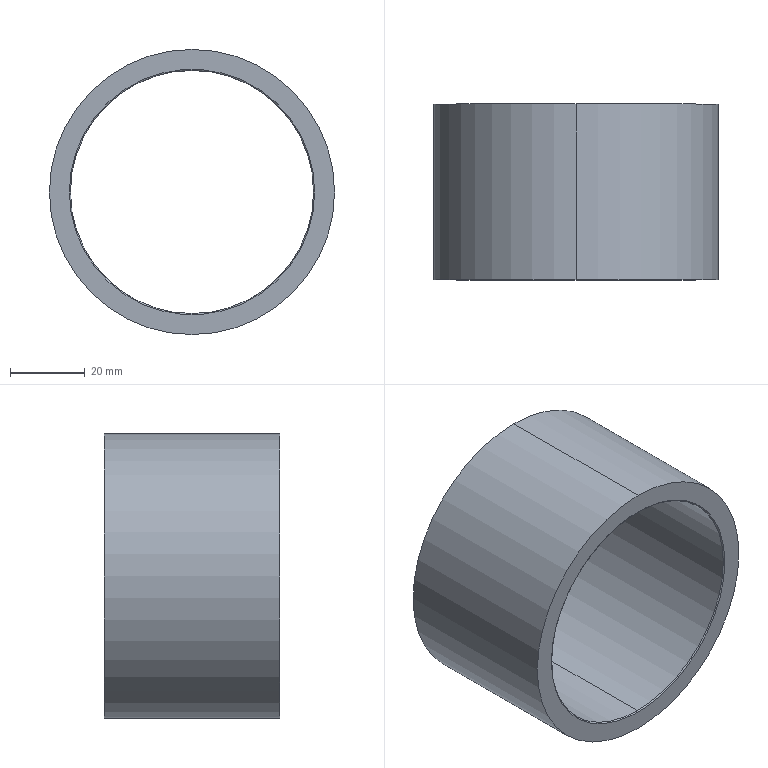Part | SolidWorks | features BaseBody 1 | 1 solid | 10 faces | box 76.25 x 47 x 76.25 mm | volume 58650 mm3 | cylinder 4 | torus 4 | plane 2 | commonest cylinder face diameters 65 x2 76.25 x2
STEP:
#1=CARTESIAN_POINT('',(-2100.15,744.069,-1577.624));
#2=VERTEX_POINT('',#1);
#3=CARTESIAN_POINT('',(-2165.75,744.069,-1577.624));
#4=VERTEX_POINT('',#3);
#5=CARTESIAN_POINT('',(-2132.95,744.069,-1577.624));
#6=DIRECTION('',(0.,-1.,0.));
#7=DIRECTION('',(0.,0.,1.));
#8=AXIS2_PLACEMENT_3D('',#5,#6,#7);
#9=CIRCLE('',#8,32.8);
#10=EDGE_CURVE('',#2,#4,#9,.T.);
#11=ORIENTED_EDGE('',*,*,#10,.F.);
#12=CARTESIAN_POINT('',(-2132.95,744.069,-1577.624));
#13=DIRECTION('',(0.,-1.,0.));
#14=DIRECTION('',(-1.,0.,0.));
#15=AXIS2_PLACEMENT_3D('',#12,#13,#14);
#16=CIRCLE('',#15,32.8);
#17=EDGE_CURVE('',#4,#2,#16,.T.);
#18=ORIENTED_EDGE('',*,*,#17,.F.);
#19=EDGE_LOOP('',(#11,#18));
#20=FACE_BOUND('',#19,.T.);
#21=CARTESIAN_POINT('',(-2132.95,744.069,-1539.499));
#22=VERTEX_POINT('',#21);
#23=CARTESIAN_POINT('',(-2132.95,744.069,-1615.749));
#24=VERTEX_POINT('',#23);
#25=CARTESIAN_POINT('',(-2132.95,744.069,-1577.624));
#26=DIRECTION('',(0.,-1.,0.));
#27=DIRECTION('',(0.,0.,1.));
#28=AXIS2_PLACEMENT_3D('',#25,#26,#27);
#29=CIRCLE('',#28,38.125);
#30=EDGE_CURVE('',#22,#24,#29,.T.);
#31=ORIENTED_EDGE('',*,*,#30,.T.);
#32=CARTESIAN_POINT('',(-2132.95,744.069,-1577.624));
#33=DIRECTION('',(0.,-1.,0.));
#34=DIRECTION('',(0.,0.,-1.));
#35=AXIS2_PLACEMENT_3D('',#32,#33,#34);
#36=CIRCLE('',#35,38.125);
#37=EDGE_CURVE('',#24,#22,#36,.T.);
#38=ORIENTED_EDGE('',*,*,#37,.T.);
#39=EDGE_LOOP('',(#31,#38));
#40=FACE_OUTER_BOUND('',#39,.T.);
#41=CARTESIAN_POINT('',(-2091.012,744.069,-1619.562));
#42=DIRECTION('',(0.,-1.,0.));
#43=DIRECTION('',(0.,0.,-1.));
#44=AXIS2_PLACEMENT_3D('',#41,#42,#43);
#45=PLANE('',#44);
#46=ADVANCED_FACE('',(#20,#40),#45,.T.);
#47=CARTESIAN_POINT('',(-2132.95,791.069,-1539.499));
#48=VERTEX_POINT('',#47);
#49=CARTESIAN_POINT('',(-2132.95,791.069,-1539.499));
#50=DIRECTION('',(0.,-1.,0.));
#51=VECTOR('',#50,1000.);
#52=LINE('',#49,#51);
#53=EDGE_CURVE('',#48,#22,#52,.T.);
#54=ORIENTED_EDGE('',*,*,#53,.T.);
#55=ORIENTED_EDGE('',*,*,#37,.F.);
#56=CARTESIAN_POINT('',(-2132.95,791.069,-1615.749));
#57=VERTEX_POINT('',#56);
#58=CARTESIAN_POINT('',(-2132.95,744.069,-1615.749));
#59=DIRECTION('',(0.,1.,0.));
#60=VECTOR('',#59,1000.);
#61=LINE('',#58,#60);
#62=EDGE_CURVE('',#24,#57,#61,.T.);
#63=ORIENTED_EDGE('',*,*,#62,.T.);
#64=CARTESIAN_POINT('',(-2132.95,791.069,-1577.624));
#65=DIRECTION('',(0.,1.,0.));
#66=DIRECTION('',(0.,0.,1.));
#67=AXIS2_PLACEMENT_3D('',#64,#65,#66);
#68=CIRCLE('',#67,38.125);
#69=EDGE_CURVE('',#48,#57,#68,.T.);
#70=ORIENTED_EDGE('',*,*,#69,.F.);
#71=EDGE_LOOP('',(#54,#55,#63,#70));
#72=FACE_OUTER_BOUND('',#71,.T.);
#73=CARTESIAN_POINT('',(-2132.95,793.419,-1577.624));
#74=DIRECTION('',(0.,1.,0.));
#75=DIRECTION('',(-0.08716,0.,0.9962));
#76=AXIS2_PLACEMENT_3D('',#73,#74,#75);
#77=CYLINDRICAL_SURFACE('',#76,38.125);
#78=ADVANCED_FACE('',(#72),#77,.T.);
#79=CARTESIAN_POINT('',(-2165.75,791.069,-1577.624));
#80=VERTEX_POINT('',#79);
#81=CARTESIAN_POINT('',(-2100.15,791.069,-1577.624));
#82=VERTEX_POINT('',#81);
#83=CARTESIAN_POINT('',(-2132.95,791.069,-1577.624));
#84=DIRECTION('',(0.,1.,0.));
#85=DIRECTION('',(-1.,0.,0.));
#86=AXIS2_PLACEMENT_3D('',#83,#84,#85);
#87=CIRCLE('',#86,32.8);
#88=EDGE_CURVE('',#80,#82,#87,.T.);
#89=ORIENTED_EDGE('',*,*,#88,.F.);
#90=CARTESIAN_POINT('',(-2132.95,791.069,-1577.624));
#91=DIRECTION('',(0.,1.,0.));
#92=DIRECTION('',(1.,0.,0.));
#93=AXIS2_PLACEMENT_3D('',#90,#91,#92);
#94=CIRCLE('',#93,32.8);
#95=EDGE_CURVE('',#82,#80,#94,.T.);
#96=ORIENTED_EDGE('',*,*,#95,.F.);
#97=EDGE_LOOP('',(#89,#96));
#98=FACE_BOUND('',#97,.T.);
#99=CARTESIAN_POINT('',(-2132.95,791.069,-1577.624));
#100=DIRECTION('',(0.,1.,0.));
#101=DIRECTION('',(0.,0.,-1.));
#102=AXIS2_PLACEMENT_3D('',#99,#100,#101);
#103=CIRCLE('',#102,38.125);
#104=EDGE_CURVE('',#57,#48,#103,.T.);
#105=ORIENTED_EDGE('',*,*,#104,.T.);
#106=ORIENTED_EDGE('',*,*,#69,.T.);
#107=EDGE_LOOP('',(#105,#106));
#108=FACE_OUTER_BOUND('',#107,.T.);
#109=CARTESIAN_POINT('',(-2091.012,791.069,-1535.687));
#110=DIRECTION('',(0.,1.,0.));
#111=DIRECTION('',(1.,0.,0.));
#112=AXIS2_PLACEMENT_3D('',#109,#110,#111);
#113=PLANE('',#112);
#114=ADVANCED_FACE('',(#98,#108),#113,.T.);
#115=CARTESIAN_POINT('',(-2100.45,790.769,-1577.624));
#116=VERTEX_POINT('',#115);
#117=CARTESIAN_POINT('',(-2100.15,790.769,-1577.624));
#118=DIRECTION('',(0.,0.,-1.));
#119=DIRECTION('',(-1.,0.,0.));
#120=AXIS2_PLACEMENT_3D('',#117,#118,#119);
#121=CIRCLE('',#120,0.3);
#122=EDGE_CURVE('',#116,#82,#121,.T.);
#123=ORIENTED_EDGE('',*,*,#122,.T.);
#124=ORIENTED_EDGE('',*,*,#95,.T.);
#125=CARTESIAN_POINT('',(-2165.45,790.769,-1577.624));
#126=VERTEX_POINT('',#125);
#127=CARTESIAN_POINT('',(-2165.75,790.769,-1577.624));
#128=DIRECTION('',(0.,0.,-1.));
#129=DIRECTION('',(0.,1.,0.));
#130=AXIS2_PLACEMENT_3D('',#127,#128,#129);
#131=CIRCLE('',#130,0.3);
#132=EDGE_CURVE('',#80,#126,#131,.T.);
#133=ORIENTED_EDGE('',*,*,#132,.T.);
#134=CARTESIAN_POINT('',(-2132.95,790.769,-1610.124));
#135=VERTEX_POINT('',#134);
#136=CARTESIAN_POINT('',(-2132.95,790.769,-1577.624));
#137=DIRECTION('',(0.,-1.,0.));
#138=DIRECTION('',(-1.,0.,0.));
#139=AXIS2_PLACEMENT_3D('',#136,#137,#138);
#140=CIRCLE('',#139,32.5);
#141=EDGE_CURVE('',#126,#135,#140,.T.);
#142=ORIENTED_EDGE('',*,*,#141,.T.);
#143=CARTESIAN_POINT('',(-2132.95,790.769,-1577.624));
#144=DIRECTION('',(0.,-1.,0.));
#145=DIRECTION('',(0.,0.,-1.));
#146=AXIS2_PLACEMENT_3D('',#143,#144,#145);
#147=CIRCLE('',#146,32.5);
#148=EDGE_CURVE('',#135,#116,#147,.T.);
#149=ORIENTED_EDGE('',*,*,#148,.T.);
#150=EDGE_LOOP('',(#123,#124,#133,#142,#149));
#151=FACE_OUTER_BOUND('',#150,.T.);
#152=CARTESIAN_POINT('',(-2132.95,790.769,-1577.624));
#153=DIRECTION('',(0.,-1.,0.));
#154=DIRECTION('',(-0.9962,0.,0.08716));
#155=AXIS2_PLACEMENT_3D('',#152,#153,#154);
#156=TOROIDAL_SURFACE('',#155,32.8,0.3);
#157=ADVANCED_FACE('',(#151),#156,.T.);
#158=CARTESIAN_POINT('',(-2132.95,790.769,-1545.124));
#159=VERTEX_POINT('',#158);
#160=CARTESIAN_POINT('',(-2132.95,744.369,-1545.124));
#161=VERTEX_POINT('',#160);
#162=CARTESIAN_POINT('',(-2132.95,790.769,-1545.124));
#163=DIRECTION('',(0.,-1.,0.));
#164=VECTOR('',#163,1000.);
#165=LINE('',#162,#164);
#166=EDGE_CURVE('',#159,#161,#165,.T.);
#167=ORIENTED_EDGE('',*,*,#166,.T.);
#168=CARTESIAN_POINT('',(-2165.45,744.369,-1577.624));
#169=VERTEX_POINT('',#168);
#170=CARTESIAN_POINT('',(-2132.95,744.369,-1577.624));
#171=DIRECTION('',(0.,-1.,0.));
#172=DIRECTION('',(0.,0.,1.));
#173=AXIS2_PLACEMENT_3D('',#170,#171,#172);
#174=CIRCLE('',#173,32.5);
#175=EDGE_CURVE('',#161,#169,#174,.T.);
#176=ORIENTED_EDGE('',*,*,#175,.T.);
#177=CARTESIAN_POINT('',(-2132.95,744.369,-1610.124));
#178=VERTEX_POINT('',#177);
#179=CARTESIAN_POINT('',(-2132.95,744.369,-1577.624));
#180=DIRECTION('',(0.,-1.,0.));
#181=DIRECTION('',(-1.,0.,0.));
#182=AXIS2_PLACEMENT_3D('',#179,#180,#181);
#183=CIRCLE('',#182,32.5);
#184=EDGE_CURVE('',#169,#178,#183,.T.);
#185=ORIENTED_EDGE('',*,*,#184,.T.);
#186=CARTESIAN_POINT('',(-2132.95,744.369,-1610.124));
#187=DIRECTION('',(0.,1.,0.));
#188=VECTOR('',#187,1000.);
#189=LINE('',#186,#188);
#190=EDGE_CURVE('',#178,#135,#189,.T.);
#191=ORIENTED_EDGE('',*,*,#190,.T.);
#192=ORIENTED_EDGE('',*,*,#141,.F.);
#193=CARTESIAN_POINT('',(-2132.95,790.769,-1577.624));
#194=DIRECTION('',(0.,-1.,0.));
#195=DIRECTION('',(0.,0.,1.));
#196=AXIS2_PLACEMENT_3D('',#193,#194,#195);
#197=CIRCLE('',#196,32.5);
#198=EDGE_CURVE('',#159,#126,#197,.T.);
#199=ORIENTED_EDGE('',*,*,#198,.F.);
#200=EDGE_LOOP('',(#167,#176,#185,#191,#192,#199));
#201=FACE_OUTER_BOUND('',#200,.T.);
#202=CARTESIAN_POINT('',(-2132.95,742.049,-1577.624));
#203=DIRECTION('',(0.,1.,0.));
#204=DIRECTION('',(0.08716,0.,-0.9962));
#205=AXIS2_PLACEMENT_3D('',#202,#203,#204);
#206=CYLINDRICAL_SURFACE('',#205,32.5);
#207=ADVANCED_FACE('',(#201),#206,.F.);
#208=CARTESIAN_POINT('',(-2100.45,744.369,-1577.624));
#209=VERTEX_POINT('',#208);
#210=CARTESIAN_POINT('',(-2100.15,744.369,-1577.624));
#211=DIRECTION('',(0.,0.,-1.));
#212=DIRECTION('',(0.,-1.,0.));
#213=AXIS2_PLACEMENT_3D('',#210,#211,#212);
#214=CIRCLE('',#213,0.3);
#215=EDGE_CURVE('',#2,#209,#214,.T.);
#216=ORIENTED_EDGE('',*,*,#215,.T.);
#217=CARTESIAN_POINT('',(-2132.95,744.369,-1577.624));
#218=DIRECTION('',(0.,-1.,0.));
#219=DIRECTION('',(0.,0.,-1.));
#220=AXIS2_PLACEMENT_3D('',#217,#218,#219);
#221=CIRCLE('',#220,32.5);
#222=EDGE_CURVE('',#178,#209,#221,.T.);
#223=ORIENTED_EDGE('',*,*,#222,.F.);
#224=ORIENTED_EDGE('',*,*,#184,.F.);
#225=CARTESIAN_POINT('',(-2165.75,744.369,-1577.624));
#226=DIRECTION('',(0.,0.,-1.));
#227=DIRECTION('',(1.,0.,0.));
#228=AXIS2_PLACEMENT_3D('',#225,#226,#227);
#229=CIRCLE('',#228,0.3);
#230=EDGE_CURVE('',#169,#4,#229,.T.);
#231=ORIENTED_EDGE('',*,*,#230,.T.);
#232=ORIENTED_EDGE('',*,*,#17,.T.);
#233=EDGE_LOOP('',(#216,#223,#224,#231,#232));
#234=FACE_OUTER_BOUND('',#233,.T.);
#235=CARTESIAN_POINT('',(-2132.95,744.369,-1577.624));
#236=DIRECTION('',(0.,-1.,0.));
#237=DIRECTION('',(-0.9962,0.,0.08716));
#238=AXIS2_PLACEMENT_3D('',#235,#236,#237);
#239=TOROIDAL_SURFACE('',#238,32.8,0.3);
#240=ADVANCED_FACE('',(#234),#239,.T.);
#241=ORIENTED_EDGE('',*,*,#215,.F.);
#242=ORIENTED_EDGE('',*,*,#10,.T.);
#243=ORIENTED_EDGE('',*,*,#230,.F.);
#244=ORIENTED_EDGE('',*,*,#175,.F.);
#245=CARTESIAN_POINT('',(-2132.95,744.369,-1577.624));
#246=DIRECTION('',(0.,-1.,0.));
#247=DIRECTION('',(1.,0.,0.));
#248=AXIS2_PLACEMENT_3D('',#245,#246,#247);
#249=CIRCLE('',#248,32.5);
#250=EDGE_CURVE('',#209,#161,#249,.T.);
#251=ORIENTED_EDGE('',*,*,#250,.F.);
#252=EDGE_LOOP('',(#241,#242,#243,#244,#251));
#253=FACE_OUTER_BOUND('',#252,.T.);
#254=CARTESIAN_POINT('',(-2132.95,744.369,-1577.624));
#255=DIRECTION('',(0.,-1.,0.));
#256=DIRECTION('',(0.9962,0.,-0.08716));
#257=AXIS2_PLACEMENT_3D('',#254,#255,#256);
#258=TOROIDAL_SURFACE('',#257,32.8,0.3);
#259=ADVANCED_FACE('',(#253),#258,.T.);
#260=ORIENTED_EDGE('',*,*,#166,.F.);
#261=CARTESIAN_POINT('',(-2132.95,790.769,-1577.624));
#262=DIRECTION('',(0.,-1.,0.));
#263=DIRECTION('',(1.,0.,0.));
#264=AXIS2_PLACEMENT_3D('',#261,#262,#263);
#265=CIRCLE('',#264,32.5);
#266=EDGE_CURVE('',#116,#159,#265,.T.);
#267=ORIENTED_EDGE('',*,*,#266,.F.);
#268=ORIENTED_EDGE('',*,*,#148,.F.);
#269=ORIENTED_EDGE('',*,*,#190,.F.);
#270=ORIENTED_EDGE('',*,*,#222,.T.);
#271=ORIENTED_EDGE('',*,*,#250,.T.);
#272=EDGE_LOOP('',(#260,#267,#268,#269,#270,#271));
#273=FACE_OUTER_BOUND('',#272,.T.);
#274=CARTESIAN_POINT('',(-2132.95,742.049,-1577.624));
#275=DIRECTION('',(0.,1.,0.));
#276=DIRECTION('',(-0.08716,0.,0.9962));
#277=AXIS2_PLACEMENT_3D('',#274,#275,#276);
#278=CYLINDRICAL_SURFACE('',#277,32.5);
#279=ADVANCED_FACE('',(#273),#278,.F.);
#280=ORIENTED_EDGE('',*,*,#122,.F.);
#281=ORIENTED_EDGE('',*,*,#266,.T.);
#282=ORIENTED_EDGE('',*,*,#198,.T.);
#283=ORIENTED_EDGE('',*,*,#132,.F.);
#284=ORIENTED_EDGE('',*,*,#88,.T.);
#285=EDGE_LOOP('',(#280,#281,#282,#283,#284));
#286=FACE_OUTER_BOUND('',#285,.T.);
#287=CARTESIAN_POINT('',(-2132.95,790.769,-1577.624));
#288=DIRECTION('',(0.,-1.,0.));
#289=DIRECTION('',(0.9962,0.,-0.08716));
#290=AXIS2_PLACEMENT_3D('',#287,#288,#289);
#291=TOROIDAL_SURFACE('',#290,32.8,0.3);
#292=ADVANCED_FACE('',(#286),#291,.T.);
#293=ORIENTED_EDGE('',*,*,#53,.F.);
#294=ORIENTED_EDGE('',*,*,#104,.F.);
#295=ORIENTED_EDGE('',*,*,#62,.F.);
#296=ORIENTED_EDGE('',*,*,#30,.F.);
#297=EDGE_LOOP('',(#293,#294,#295,#296));
#298=FACE_OUTER_BOUND('',#297,.T.);
#299=CARTESIAN_POINT('',(-2132.95,793.419,-1577.624));
#300=DIRECTION('',(0.,1.,0.));
#301=DIRECTION('',(0.08716,0.,-0.9962));
#302=AXIS2_PLACEMENT_3D('',#299,#300,#301);
#303=CYLINDRICAL_SURFACE('',#302,38.125);
#304=ADVANCED_FACE('',(#298),#303,.T.);
#305=CLOSED_SHELL('',(#46,#78,#114,#157,#207,#240,#259,#279,#292,#304));
#306=MANIFOLD_SOLID_BREP('',#305);
#307=CARTESIAN_POINT('',(0.,0.,0.));
#308=DIRECTION('',(0.,0.,1.));
#309=DIRECTION('',(1.,0.,0.));
#310=AXIS2_PLACEMENT_3D('',#307,#308,#309);
#311=(LENGTH_UNIT()NAMED_UNIT(*)SI_UNIT(.MILLI.,.METRE.));
#312=UNCERTAINTY_MEASURE_WITH_UNIT(LENGTH_MEASURE(0.00001),#311,'','');
#313=(NAMED_UNIT(*)PLANE_ANGLE_UNIT()SI_UNIT($,.RADIAN.));
#314=(NAMED_UNIT(*)SI_UNIT($,.STERADIAN.)SOLID_ANGLE_UNIT());
#315=(GEOMETRIC_REPRESENTATION_CONTEXT(3)GLOBAL_UNCERTAINTY_ASSIGNED_CONTEXT((#312))GLOBAL_UNIT_ASSIGNED_CONTEXT((#311,#313,#314))REPRESENTATION_CONTEXT('',''));
#316=ADVANCED_BREP_SHAPE_REPRESENTATION('',(#306,#310),#315);